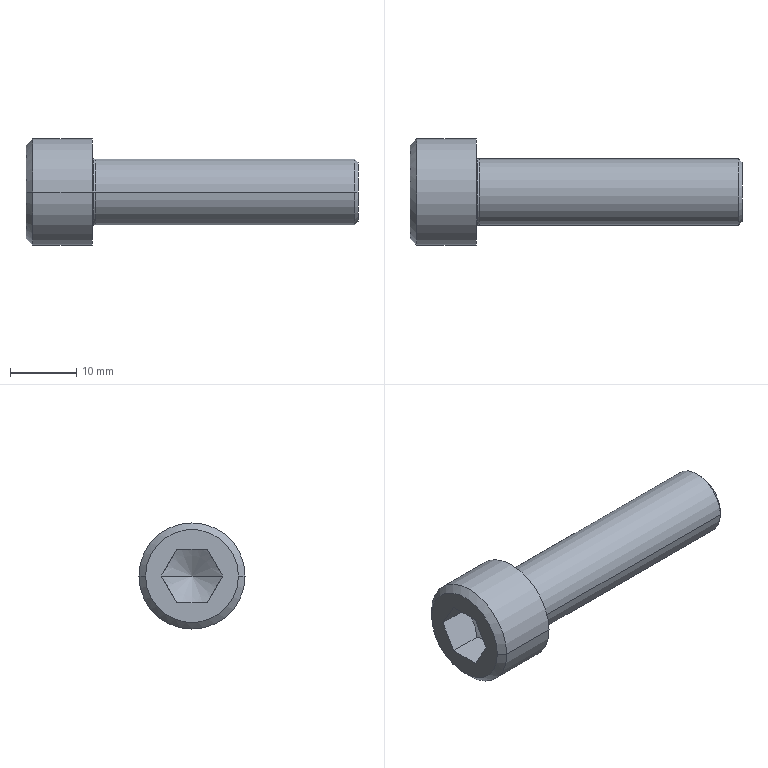Part | Creo | 1 solid | 23 faces | box 50 x 16 x 16 mm | volume 4790 mm3 | plane 9 | cone 6 | cylinder 4 | torus 4 | commonest cylinder face diameters 10 x2 16 x2
STEP:
#1=CARTESIAN_POINT('',(-308.5,10.376,-111.));
#2=VERTEX_POINT('',#1);
#3=CARTESIAN_POINT('',(-308.5,12.686,-107.));
#4=VERTEX_POINT('',#3);
#5=CARTESIAN_POINT('',(-308.5,10.376,-111.));
#6=CARTESIAN_POINT('',(-308.438,10.484,-110.814));
#7=CARTESIAN_POINT('',(-308.326,10.7,-110.439));
#8=CARTESIAN_POINT('',(-308.205,11.03,-109.869));
#9=CARTESIAN_POINT('',(-308.14,11.363,-109.291));
#10=CARTESIAN_POINT('',(-308.14,11.698,-108.712));
#11=CARTESIAN_POINT('',(-308.204,12.032,-108.133));
#12=CARTESIAN_POINT('',(-308.325,12.361,-107.563));
#13=CARTESIAN_POINT('',(-308.438,12.578,-107.187));
#14=CARTESIAN_POINT('',(-308.5,12.686,-107.));
#15=B_SPLINE_CURVE_WITH_KNOTS('',3,(#5,#6,#7,#8,#9,#10,#11,#12,#13,#14),.UNSPECIFIED.,.F.,.F.,(4,1,1,1,1,1,1,4),(0.,0.1429,0.2857,0.4286,0.5714,0.7143,0.8571,1.),.UNSPECIFIED.);
#16=EDGE_CURVE('',#2,#4,#15,.T.);
#17=ORIENTED_EDGE('',*,*,#16,.F.);
#18=CARTESIAN_POINT('',(-305.833,14.995,-111.));
#19=VERTEX_POINT('',#18);
#20=CARTESIAN_POINT('',(-305.833,14.995,-111.));
#21=DIRECTION('',(-0.5,-0.866,0.));
#22=VECTOR('',#21,5.333);
#23=LINE('',#20,#22);
#24=EDGE_CURVE('',#19,#2,#23,.T.);
#25=ORIENTED_EDGE('',*,*,#24,.F.);
#26=CARTESIAN_POINT('',(-308.5,19.614,-111.));
#27=VERTEX_POINT('',#26);
#28=CARTESIAN_POINT('',(-305.833,14.995,-111.));
#29=DIRECTION('',(-0.5,0.866,0.));
#30=VECTOR('',#29,5.333);
#31=LINE('',#28,#30);
#32=EDGE_CURVE('',#19,#27,#31,.T.);
#33=ORIENTED_EDGE('',*,*,#32,.T.);
#34=CARTESIAN_POINT('',(-308.5,17.305,-107.));
#35=VERTEX_POINT('',#34);
#36=CARTESIAN_POINT('',(-308.5,17.305,-107.));
#37=CARTESIAN_POINT('',(-308.438,17.412,-107.186));
#38=CARTESIAN_POINT('',(-308.326,17.628,-107.561));
#39=CARTESIAN_POINT('',(-308.205,17.958,-108.131));
#40=CARTESIAN_POINT('',(-308.14,18.291,-108.709));
#41=CARTESIAN_POINT('',(-308.14,18.626,-109.288));
#42=CARTESIAN_POINT('',(-308.204,18.96,-109.867));
#43=CARTESIAN_POINT('',(-308.325,19.289,-110.437));
#44=CARTESIAN_POINT('',(-308.438,19.506,-110.813));
#45=CARTESIAN_POINT('',(-308.5,19.614,-111.));
#46=B_SPLINE_CURVE_WITH_KNOTS('',3,(#36,#37,#38,#39,#40,#41,#42,#43,#44,#45),.UNSPECIFIED.,.F.,.F.,(4,1,1,1,1,1,1,4),(0.,0.1429,0.2857,0.4286,0.5714,0.7143,0.8571,1.),.UNSPECIFIED.);
#47=EDGE_CURVE('',#35,#27,#46,.T.);
#48=ORIENTED_EDGE('',*,*,#47,.F.);
#49=CARTESIAN_POINT('',(-308.5,12.686,-107.));
#50=CARTESIAN_POINT('',(-308.438,12.9,-107.));
#51=CARTESIAN_POINT('',(-308.327,13.33,-107.));
#52=CARTESIAN_POINT('',(-308.205,13.992,-107.));
#53=CARTESIAN_POINT('',(-308.14,14.66,-107.));
#54=CARTESIAN_POINT('',(-308.14,15.328,-107.));
#55=CARTESIAN_POINT('',(-308.204,15.996,-107.));
#56=CARTESIAN_POINT('',(-308.326,16.657,-107.));
#57=CARTESIAN_POINT('',(-308.438,17.09,-107.));
#58=CARTESIAN_POINT('',(-308.5,17.305,-107.));
#59=B_SPLINE_CURVE_WITH_KNOTS('',3,(#49,#50,#51,#52,#53,#54,#55,#56,#57,#58),.UNSPECIFIED.,.F.,.F.,(4,1,1,1,1,1,1,4),(0.,0.1429,0.2857,0.4286,0.5714,0.7143,0.8571,1.),.UNSPECIFIED.);
#60=EDGE_CURVE('',#4,#35,#59,.T.);
#61=ORIENTED_EDGE('',*,*,#60,.F.);
#62=EDGE_LOOP('',(#17,#25,#33,#48,#61));
#63=FACE_OUTER_BOUND('',#62,.F.);
#64=CARTESIAN_POINT('',(-307.193,14.995,-111.));
#65=DIRECTION('',(-1.,0.,0.));
#66=DIRECTION('',(0.,-1.,0.));
#67=AXIS2_PLACEMENT_3D('',#64,#65,#66);
#68=CONICAL_SURFACE('',#67,2.356,60.);
#69=ADVANCED_FACE('',(#63),#68,.F.);
#70=CARTESIAN_POINT('',(-313.5,12.686,-107.));
#71=VERTEX_POINT('',#70);
#72=CARTESIAN_POINT('',(-313.5,10.376,-111.));
#73=VERTEX_POINT('',#72);
#74=CARTESIAN_POINT('',(-313.5,12.686,-107.));
#75=DIRECTION('',(0.,-0.5,-0.866));
#76=VECTOR('',#75,4.619);
#77=LINE('',#74,#76);
#78=EDGE_CURVE('',#71,#73,#77,.T.);
#79=ORIENTED_EDGE('',*,*,#78,.T.);
#80=CARTESIAN_POINT('',(-313.5,10.376,-111.));
#81=DIRECTION('',(1.,0.,0.));
#82=VECTOR('',#81,5.);
#83=LINE('',#80,#82);
#84=EDGE_CURVE('',#73,#2,#83,.T.);
#85=ORIENTED_EDGE('',*,*,#84,.T.);
#86=ORIENTED_EDGE('',*,*,#16,.T.);
#87=CARTESIAN_POINT('',(-313.5,12.686,-107.));
#88=DIRECTION('',(1.,0.,0.));
#89=VECTOR('',#88,5.);
#90=LINE('',#87,#89);
#91=EDGE_CURVE('',#71,#4,#90,.T.);
#92=ORIENTED_EDGE('',*,*,#91,.F.);
#93=EDGE_LOOP('',(#79,#85,#86,#92));
#94=FACE_OUTER_BOUND('',#93,.F.);
#95=CARTESIAN_POINT('',(-308.5,12.686,-107.));
#96=DIRECTION('',(0.,0.866,-0.5));
#97=DIRECTION('',(0.,-0.5,-0.866));
#98=AXIS2_PLACEMENT_3D('',#95,#96,#97);
#99=PLANE('',#98);
#100=ADVANCED_FACE('',(#94),#99,.T.);
#101=CARTESIAN_POINT('',(-313.5,7.995,-111.));
#102=VERTEX_POINT('',#101);
#103=CARTESIAN_POINT('',(-313.5,21.995,-111.));
#104=VERTEX_POINT('',#103);
#105=CARTESIAN_POINT('',(-313.5,14.995,-111.));
#106=DIRECTION('',(-1.,0.,0.));
#107=DIRECTION('',(0.,-1.,0.));
#108=AXIS2_PLACEMENT_3D('',#105,#106,#107);
#109=CIRCLE('',#108,7.);
#110=EDGE_CURVE('',#102,#104,#109,.T.);
#111=ORIENTED_EDGE('',*,*,#110,.F.);
#112=CARTESIAN_POINT('',(-313.5,14.995,-111.));
#113=DIRECTION('',(-1.,0.,0.));
#114=DIRECTION('',(0.,1.,0.));
#115=AXIS2_PLACEMENT_3D('',#112,#113,#114);
#116=CIRCLE('',#115,7.);
#117=EDGE_CURVE('',#104,#102,#116,.T.);
#118=ORIENTED_EDGE('',*,*,#117,.F.);
#119=EDGE_LOOP('',(#111,#118));
#120=FACE_OUTER_BOUND('',#119,.F.);
#121=CARTESIAN_POINT('',(-313.5,12.686,-115.));
#122=VERTEX_POINT('',#121);
#123=CARTESIAN_POINT('',(-313.5,10.376,-111.));
#124=DIRECTION('',(0.,0.5,-0.866));
#125=VECTOR('',#124,4.619);
#126=LINE('',#123,#125);
#127=EDGE_CURVE('',#73,#122,#126,.T.);
#128=ORIENTED_EDGE('',*,*,#127,.F.);
#129=ORIENTED_EDGE('',*,*,#78,.F.);
#130=CARTESIAN_POINT('',(-313.5,17.305,-107.));
#131=VERTEX_POINT('',#130);
#132=CARTESIAN_POINT('',(-313.5,12.686,-107.));
#133=DIRECTION('',(0.,1.,0.));
#134=VECTOR('',#133,4.619);
#135=LINE('',#132,#134);
#136=EDGE_CURVE('',#71,#131,#135,.T.);
#137=ORIENTED_EDGE('',*,*,#136,.T.);
#138=CARTESIAN_POINT('',(-313.5,19.614,-111.));
#139=VERTEX_POINT('',#138);
#140=CARTESIAN_POINT('',(-313.5,19.614,-111.));
#141=DIRECTION('',(0.,-0.5,0.866));
#142=VECTOR('',#141,4.619);
#143=LINE('',#140,#142);
#144=EDGE_CURVE('',#139,#131,#143,.T.);
#145=ORIENTED_EDGE('',*,*,#144,.F.);
#146=CARTESIAN_POINT('',(-313.5,17.305,-115.));
#147=VERTEX_POINT('',#146);
#148=CARTESIAN_POINT('',(-313.5,17.305,-115.));
#149=DIRECTION('',(0.,0.5,0.866));
#150=VECTOR('',#149,4.619);
#151=LINE('',#148,#150);
#152=EDGE_CURVE('',#147,#139,#151,.T.);
#153=ORIENTED_EDGE('',*,*,#152,.F.);
#154=CARTESIAN_POINT('',(-313.5,17.305,-115.));
#155=DIRECTION('',(0.,-1.,0.));
#156=VECTOR('',#155,4.619);
#157=LINE('',#154,#156);
#158=EDGE_CURVE('',#147,#122,#157,.T.);
#159=ORIENTED_EDGE('',*,*,#158,.T.);
#160=EDGE_LOOP('',(#128,#129,#137,#145,#153,#159));
#161=FACE_BOUND('',#160,.F.);
#162=CARTESIAN_POINT('',(-313.5,14.995,-111.));
#163=DIRECTION('',(-1.,0.,0.));
#164=DIRECTION('',(0.,-1.,0.));
#165=AXIS2_PLACEMENT_3D('',#162,#163,#164);
#166=PLANE('',#165);
#167=ADVANCED_FACE('',(#120,#161),#166,.T.);
#168=CARTESIAN_POINT('',(-312.5,6.995,-111.));
#169=VERTEX_POINT('',#168);
#170=CARTESIAN_POINT('',(-312.5,22.995,-111.));
#171=VERTEX_POINT('',#170);
#172=CARTESIAN_POINT('',(-312.5,14.995,-111.));
#173=DIRECTION('',(-1.,0.,0.));
#174=DIRECTION('',(0.,-1.,0.));
#175=AXIS2_PLACEMENT_3D('',#172,#173,#174);
#176=CIRCLE('',#175,8.);
#177=EDGE_CURVE('',#169,#171,#176,.T.);
#178=ORIENTED_EDGE('',*,*,#177,.F.);
#179=CARTESIAN_POINT('',(-313.5,7.995,-111.));
#180=DIRECTION('',(0.7071,-0.7071,0.));
#181=VECTOR('',#180,1.414);
#182=LINE('',#179,#181);
#183=EDGE_CURVE('',#102,#169,#182,.T.);
#184=ORIENTED_EDGE('',*,*,#183,.F.);
#185=ORIENTED_EDGE('',*,*,#110,.T.);
#186=CARTESIAN_POINT('',(-313.5,21.995,-111.));
#187=DIRECTION('',(0.7071,0.7071,0.));
#188=VECTOR('',#187,1.414);
#189=LINE('',#186,#188);
#190=EDGE_CURVE('',#104,#171,#189,.T.);
#191=ORIENTED_EDGE('',*,*,#190,.T.);
#192=EDGE_LOOP('',(#178,#184,#185,#191));
#193=FACE_OUTER_BOUND('',#192,.F.);
#194=CARTESIAN_POINT('',(-313.,14.995,-111.));
#195=DIRECTION('',(1.,0.,0.));
#196=DIRECTION('',(0.,1.,0.));
#197=AXIS2_PLACEMENT_3D('',#194,#195,#196);
#198=CONICAL_SURFACE('',#197,7.5,45.);
#199=ADVANCED_FACE('',(#193),#198,.T.);
#200=ORIENTED_EDGE('',*,*,#177,.T.);
#201=CARTESIAN_POINT('',(-303.5,22.995,-111.));
#202=VERTEX_POINT('',#201);
#203=CARTESIAN_POINT('',(-303.5,22.995,-111.));
#204=DIRECTION('',(-1.,0.,0.));
#205=VECTOR('',#204,9.);
#206=LINE('',#203,#205);
#207=EDGE_CURVE('',#202,#171,#206,.T.);
#208=ORIENTED_EDGE('',*,*,#207,.F.);
#209=CARTESIAN_POINT('',(-303.5,6.995,-111.));
#210=VERTEX_POINT('',#209);
#211=CARTESIAN_POINT('',(-303.5,14.995,-111.));
#212=DIRECTION('',(1.,0.,0.));
#213=DIRECTION('',(0.,1.,0.));
#214=AXIS2_PLACEMENT_3D('',#211,#212,#213);
#215=CIRCLE('',#214,8.);
#216=EDGE_CURVE('',#202,#210,#215,.T.);
#217=ORIENTED_EDGE('',*,*,#216,.T.);
#218=CARTESIAN_POINT('',(-303.5,6.995,-111.));
#219=DIRECTION('',(-1.,0.,0.));
#220=VECTOR('',#219,9.);
#221=LINE('',#218,#220);
#222=EDGE_CURVE('',#210,#169,#221,.T.);
#223=ORIENTED_EDGE('',*,*,#222,.T.);
#224=EDGE_LOOP('',(#200,#208,#217,#223));
#225=FACE_OUTER_BOUND('',#224,.F.);
#226=CARTESIAN_POINT('',(-303.5,14.995,-111.));
#227=DIRECTION('',(-1.,0.,0.));
#228=DIRECTION('',(0.,-1.,0.));
#229=AXIS2_PLACEMENT_3D('',#226,#227,#228);
#230=CYLINDRICAL_SURFACE('',#229,8.);
#231=ADVANCED_FACE('',(#225),#230,.T.);
#232=CARTESIAN_POINT('',(-312.5,14.995,-111.));
#233=DIRECTION('',(-1.,0.,0.));
#234=DIRECTION('',(0.,1.,0.));
#235=AXIS2_PLACEMENT_3D('',#232,#233,#234);
#236=CIRCLE('',#235,8.);
#237=EDGE_CURVE('',#171,#169,#236,.T.);
#238=ORIENTED_EDGE('',*,*,#237,.T.);
#239=ORIENTED_EDGE('',*,*,#222,.F.);
#240=CARTESIAN_POINT('',(-303.5,14.995,-111.));
#241=DIRECTION('',(1.,0.,0.));
#242=DIRECTION('',(0.,-1.,0.));
#243=AXIS2_PLACEMENT_3D('',#240,#241,#242);
#244=CIRCLE('',#243,8.);
#245=EDGE_CURVE('',#210,#202,#244,.T.);
#246=ORIENTED_EDGE('',*,*,#245,.T.);
#247=ORIENTED_EDGE('',*,*,#207,.T.);
#248=EDGE_LOOP('',(#238,#239,#246,#247));
#249=FACE_OUTER_BOUND('',#248,.F.);
#250=CARTESIAN_POINT('',(-303.5,14.995,-111.));
#251=DIRECTION('',(-1.,0.,0.));
#252=DIRECTION('',(0.,-1.,0.));
#253=AXIS2_PLACEMENT_3D('',#250,#251,#252);
#254=CYLINDRICAL_SURFACE('',#253,8.);
#255=ADVANCED_FACE('',(#249),#254,.T.);
#256=ORIENTED_EDGE('',*,*,#237,.F.);
#257=ORIENTED_EDGE('',*,*,#190,.F.);
#258=ORIENTED_EDGE('',*,*,#117,.T.);
#259=ORIENTED_EDGE('',*,*,#183,.T.);
#260=EDGE_LOOP('',(#256,#257,#258,#259));
#261=FACE_OUTER_BOUND('',#260,.F.);
#262=CARTESIAN_POINT('',(-313.,14.995,-111.));
#263=DIRECTION('',(1.,0.,0.));
#264=DIRECTION('',(0.,1.,0.));
#265=AXIS2_PLACEMENT_3D('',#262,#263,#264);
#266=CONICAL_SURFACE('',#265,7.5,45.);
#267=ADVANCED_FACE('',(#261),#266,.T.);
#268=ORIENTED_EDGE('',*,*,#245,.F.);
#269=ORIENTED_EDGE('',*,*,#216,.F.);
#270=EDGE_LOOP('',(#268,#269));
#271=FACE_OUTER_BOUND('',#270,.F.);
#272=CARTESIAN_POINT('',(-303.5,9.595,-111.));
#273=VERTEX_POINT('',#272);
#274=CARTESIAN_POINT('',(-303.5,20.395,-111.));
#275=VERTEX_POINT('',#274);
#276=CARTESIAN_POINT('',(-303.5,14.995,-111.));
#277=DIRECTION('',(-1.,0.,0.));
#278=DIRECTION('',(0.,-1.,0.));
#279=AXIS2_PLACEMENT_3D('',#276,#277,#278);
#280=CIRCLE('',#279,5.4);
#281=EDGE_CURVE('',#273,#275,#280,.T.);
#282=ORIENTED_EDGE('',*,*,#281,.F.);
#283=CARTESIAN_POINT('',(-303.5,14.995,-111.));
#284=DIRECTION('',(-1.,0.,0.));
#285=DIRECTION('',(0.,1.,0.));
#286=AXIS2_PLACEMENT_3D('',#283,#284,#285);
#287=CIRCLE('',#286,5.4);
#288=EDGE_CURVE('',#275,#273,#287,.T.);
#289=ORIENTED_EDGE('',*,*,#288,.F.);
#290=EDGE_LOOP('',(#282,#289));
#291=FACE_BOUND('',#290,.F.);
#292=CARTESIAN_POINT('',(-303.5,14.995,-111.));
#293=DIRECTION('',(-1.,0.,0.));
#294=DIRECTION('',(0.,-1.,0.));
#295=AXIS2_PLACEMENT_3D('',#292,#293,#294);
#296=PLANE('',#295);
#297=ADVANCED_FACE('',(#271,#291),#296,.F.);
#298=ORIENTED_EDGE('',*,*,#281,.T.);
#299=CARTESIAN_POINT('',(-303.383,20.112,-111.));
#300=VERTEX_POINT('',#299);
#301=CARTESIAN_POINT('',(-303.1,20.395,-111.));
#302=DIRECTION('',(0.,0.,1.));
#303=DIRECTION('',(-1.,0.,0.));
#304=AXIS2_PLACEMENT_3D('',#301,#302,#303);
#305=CIRCLE('',#304,0.4);
#306=EDGE_CURVE('',#275,#300,#305,.T.);
#307=ORIENTED_EDGE('',*,*,#306,.T.);
#308=CARTESIAN_POINT('',(-303.383,9.878,-111.));
#309=VERTEX_POINT('',#308);
#310=CARTESIAN_POINT('',(-303.383,14.995,-111.));
#311=DIRECTION('',(-1.,0.,0.));
#312=DIRECTION('',(0.,-1.,0.));
#313=AXIS2_PLACEMENT_3D('',#310,#311,#312);
#314=CIRCLE('',#313,5.117);
#315=EDGE_CURVE('',#309,#300,#314,.T.);
#316=ORIENTED_EDGE('',*,*,#315,.F.);
#317=CARTESIAN_POINT('',(-303.1,9.595,-111.));
#318=DIRECTION('',(0.,0.,-1.));
#319=DIRECTION('',(-1.,0.,0.));
#320=AXIS2_PLACEMENT_3D('',#317,#318,#319);
#321=CIRCLE('',#320,0.4);
#322=EDGE_CURVE('',#273,#309,#321,.T.);
#323=ORIENTED_EDGE('',*,*,#322,.F.);
#324=EDGE_LOOP('',(#298,#307,#316,#323));
#325=FACE_OUTER_BOUND('',#324,.F.);
#326=CARTESIAN_POINT('',(-303.1,14.995,-111.));
#327=DIRECTION('',(-1.,0.,0.));
#328=DIRECTION('',(0.,-1.,0.));
#329=AXIS2_PLACEMENT_3D('',#326,#327,#328);
#330=TOROIDAL_SURFACE('',#329,5.4,0.4);
#331=ADVANCED_FACE('',(#325),#330,.F.);
#332=ORIENTED_EDGE('',*,*,#288,.T.);
#333=ORIENTED_EDGE('',*,*,#322,.T.);
#334=CARTESIAN_POINT('',(-303.383,14.995,-111.));
#335=DIRECTION('',(-1.,0.,0.));
#336=DIRECTION('',(0.,1.,0.));
#337=AXIS2_PLACEMENT_3D('',#334,#335,#336);
#338=CIRCLE('',#337,5.117);
#339=EDGE_CURVE('',#300,#309,#338,.T.);
#340=ORIENTED_EDGE('',*,*,#339,.F.);
#341=ORIENTED_EDGE('',*,*,#306,.F.);
#342=EDGE_LOOP('',(#332,#333,#340,#341));
#343=FACE_OUTER_BOUND('',#342,.F.);
#344=CARTESIAN_POINT('',(-303.1,14.995,-111.));
#345=DIRECTION('',(-1.,0.,0.));
#346=DIRECTION('',(0.,-1.,0.));
#347=AXIS2_PLACEMENT_3D('',#344,#345,#346);
#348=TOROIDAL_SURFACE('',#347,5.4,0.4);
#349=ADVANCED_FACE('',(#343),#348,.F.);
#350=CARTESIAN_POINT('',(-303.1,19.995,-111.));
#351=VERTEX_POINT('',#350);
#352=CARTESIAN_POINT('',(-303.1,9.995,-111.));
#353=VERTEX_POINT('',#352);
#354=CARTESIAN_POINT('',(-303.1,14.995,-111.));
#355=DIRECTION('',(-1.,0.,0.));
#356=DIRECTION('',(0.,1.,0.));
#357=AXIS2_PLACEMENT_3D('',#354,#355,#356);
#358=CIRCLE('',#357,5.);
#359=EDGE_CURVE('',#351,#353,#358,.T.);
#360=ORIENTED_EDGE('',*,*,#359,.F.);
#361=CARTESIAN_POINT('',(-303.1,20.395,-111.));
#362=DIRECTION('',(0.,0.,1.));
#363=DIRECTION('',(-0.7071,-0.7071,0.));
#364=AXIS2_PLACEMENT_3D('',#361,#362,#363);
#365=CIRCLE('',#364,0.4);
#366=EDGE_CURVE('',#300,#351,#365,.T.);
#367=ORIENTED_EDGE('',*,*,#366,.F.);
#368=ORIENTED_EDGE('',*,*,#339,.T.);
#369=CARTESIAN_POINT('',(-303.1,9.595,-111.));
#370=DIRECTION('',(0.,0.,-1.));
#371=DIRECTION('',(-0.7071,0.7071,0.));
#372=AXIS2_PLACEMENT_3D('',#369,#370,#371);
#373=CIRCLE('',#372,0.4);
#374=EDGE_CURVE('',#309,#353,#373,.T.);
#375=ORIENTED_EDGE('',*,*,#374,.T.);
#376=EDGE_LOOP('',(#360,#367,#368,#375));
#377=FACE_OUTER_BOUND('',#376,.F.);
#378=CARTESIAN_POINT('',(-303.1,14.995,-111.));
#379=DIRECTION('',(-1.,0.,0.));
#380=DIRECTION('',(0.,-1.,0.));
#381=AXIS2_PLACEMENT_3D('',#378,#379,#380);
#382=TOROIDAL_SURFACE('',#381,5.4,0.4);
#383=ADVANCED_FACE('',(#377),#382,.F.);
#384=CARTESIAN_POINT('',(-264.,9.995,-111.));
#385=VERTEX_POINT('',#384);
#386=CARTESIAN_POINT('',(-264.,19.995,-111.));
#387=VERTEX_POINT('',#386);
#388=CARTESIAN_POINT('',(-264.,14.995,-111.));
#389=DIRECTION('',(1.,0.,0.));
#390=DIRECTION('',(0.,-1.,0.));
#391=AXIS2_PLACEMENT_3D('',#388,#389,#390);
#392=CIRCLE('',#391,5.);
#393=EDGE_CURVE('',#385,#387,#392,.T.);
#394=ORIENTED_EDGE('',*,*,#393,.T.);
#395=CARTESIAN_POINT('',(-264.,19.995,-111.));
#396=DIRECTION('',(-1.,0.,0.));
#397=VECTOR('',#396,39.1);
#398=LINE('',#395,#397);
#399=EDGE_CURVE('',#387,#351,#398,.T.);
#400=ORIENTED_EDGE('',*,*,#399,.T.);
#401=ORIENTED_EDGE('',*,*,#359,.T.);
#402=CARTESIAN_POINT('',(-264.,9.995,-111.));
#403=DIRECTION('',(-1.,0.,0.));
#404=VECTOR('',#403,39.1);
#405=LINE('',#402,#404);
#406=EDGE_CURVE('',#385,#353,#405,.T.);
#407=ORIENTED_EDGE('',*,*,#406,.F.);
#408=EDGE_LOOP('',(#394,#400,#401,#407));
#409=FACE_OUTER_BOUND('',#408,.F.);
#410=CARTESIAN_POINT('',(-263.5,14.995,-111.));
#411=DIRECTION('',(-1.,0.,0.));
#412=DIRECTION('',(0.,-1.,0.));
#413=AXIS2_PLACEMENT_3D('',#410,#411,#412);
#414=CYLINDRICAL_SURFACE('',#413,5.);
#415=ADVANCED_FACE('',(#409),#414,.T.);
#416=CARTESIAN_POINT('',(-263.5,10.495,-111.));
#417=VERTEX_POINT('',#416);
#418=CARTESIAN_POINT('',(-263.5,19.495,-111.));
#419=VERTEX_POINT('',#418);
#420=CARTESIAN_POINT('',(-263.5,14.995,-111.));
#421=DIRECTION('',(1.,0.,0.));
#422=DIRECTION('',(0.,-1.,0.));
#423=AXIS2_PLACEMENT_3D('',#420,#421,#422);
#424=CIRCLE('',#423,4.5);
#425=EDGE_CURVE('',#417,#419,#424,.T.);
#426=ORIENTED_EDGE('',*,*,#425,.T.);
#427=CARTESIAN_POINT('',(-263.5,19.495,-111.));
#428=DIRECTION('',(-0.7071,0.7071,0.));
#429=VECTOR('',#428,0.7071);
#430=LINE('',#427,#429);
#431=EDGE_CURVE('',#419,#387,#430,.T.);
#432=ORIENTED_EDGE('',*,*,#431,.T.);
#433=ORIENTED_EDGE('',*,*,#393,.F.);
#434=CARTESIAN_POINT('',(-263.5,10.495,-111.));
#435=DIRECTION('',(-0.7071,-0.7071,0.));
#436=VECTOR('',#435,0.7071);
#437=LINE('',#434,#436);
#438=EDGE_CURVE('',#417,#385,#437,.T.);
#439=ORIENTED_EDGE('',*,*,#438,.F.);
#440=EDGE_LOOP('',(#426,#432,#433,#439));
#441=FACE_OUTER_BOUND('',#440,.F.);
#442=CARTESIAN_POINT('',(-263.75,14.995,-111.));
#443=DIRECTION('',(-1.,0.,0.));
#444=DIRECTION('',(0.,-1.,0.));
#445=AXIS2_PLACEMENT_3D('',#442,#443,#444);
#446=CONICAL_SURFACE('',#445,4.75,45.);
#447=ADVANCED_FACE('',(#441),#446,.T.);
#448=ORIENTED_EDGE('',*,*,#425,.F.);
#449=CARTESIAN_POINT('',(-263.5,14.995,-111.));
#450=DIRECTION('',(1.,0.,0.));
#451=DIRECTION('',(0.,1.,0.));
#452=AXIS2_PLACEMENT_3D('',#449,#450,#451);
#453=CIRCLE('',#452,4.5);
#454=EDGE_CURVE('',#419,#417,#453,.T.);
#455=ORIENTED_EDGE('',*,*,#454,.F.);
#456=EDGE_LOOP('',(#448,#455));
#457=FACE_OUTER_BOUND('',#456,.F.);
#458=CARTESIAN_POINT('',(-263.5,14.995,-111.));
#459=DIRECTION('',(-1.,0.,0.));
#460=DIRECTION('',(0.,-1.,0.));
#461=AXIS2_PLACEMENT_3D('',#458,#459,#460);
#462=PLANE('',#461);
#463=ADVANCED_FACE('',(#457),#462,.F.);
#464=ORIENTED_EDGE('',*,*,#454,.T.);
#465=ORIENTED_EDGE('',*,*,#438,.T.);
#466=CARTESIAN_POINT('',(-264.,14.995,-111.));
#467=DIRECTION('',(1.,0.,0.));
#468=DIRECTION('',(0.,1.,0.));
#469=AXIS2_PLACEMENT_3D('',#466,#467,#468);
#470=CIRCLE('',#469,5.);
#471=EDGE_CURVE('',#387,#385,#470,.T.);
#472=ORIENTED_EDGE('',*,*,#471,.F.);
#473=ORIENTED_EDGE('',*,*,#431,.F.);
#474=EDGE_LOOP('',(#464,#465,#472,#473));
#475=FACE_OUTER_BOUND('',#474,.F.);
#476=CARTESIAN_POINT('',(-263.75,14.995,-111.));
#477=DIRECTION('',(-1.,0.,0.));
#478=DIRECTION('',(0.,-1.,0.));
#479=AXIS2_PLACEMENT_3D('',#476,#477,#478);
#480=CONICAL_SURFACE('',#479,4.75,45.);
#481=ADVANCED_FACE('',(#475),#480,.T.);
#482=ORIENTED_EDGE('',*,*,#471,.T.);
#483=ORIENTED_EDGE('',*,*,#406,.T.);
#484=CARTESIAN_POINT('',(-303.1,14.995,-111.));
#485=DIRECTION('',(-1.,0.,0.));
#486=DIRECTION('',(0.,-1.,0.));
#487=AXIS2_PLACEMENT_3D('',#484,#485,#486);
#488=CIRCLE('',#487,5.);
#489=EDGE_CURVE('',#353,#351,#488,.T.);
#490=ORIENTED_EDGE('',*,*,#489,.T.);
#491=ORIENTED_EDGE('',*,*,#399,.F.);
#492=EDGE_LOOP('',(#482,#483,#490,#491));
#493=FACE_OUTER_BOUND('',#492,.F.);
#494=CARTESIAN_POINT('',(-263.5,14.995,-111.));
#495=DIRECTION('',(-1.,0.,0.));
#496=DIRECTION('',(0.,-1.,0.));
#497=AXIS2_PLACEMENT_3D('',#494,#495,#496);
#498=CYLINDRICAL_SURFACE('',#497,5.);
#499=ADVANCED_FACE('',(#493),#498,.T.);
#500=ORIENTED_EDGE('',*,*,#489,.F.);
#501=ORIENTED_EDGE('',*,*,#374,.F.);
#502=ORIENTED_EDGE('',*,*,#315,.T.);
#503=ORIENTED_EDGE('',*,*,#366,.T.);
#504=EDGE_LOOP('',(#500,#501,#502,#503));
#505=FACE_OUTER_BOUND('',#504,.F.);
#506=CARTESIAN_POINT('',(-303.1,14.995,-111.));
#507=DIRECTION('',(-1.,0.,0.));
#508=DIRECTION('',(0.,-1.,0.));
#509=AXIS2_PLACEMENT_3D('',#506,#507,#508);
#510=TOROIDAL_SURFACE('',#509,5.4,0.4);
#511=ADVANCED_FACE('',(#505),#510,.F.);
#512=ORIENTED_EDGE('',*,*,#127,.T.);
#513=CARTESIAN_POINT('',(-308.5,12.686,-115.));
#514=VERTEX_POINT('',#513);
#515=CARTESIAN_POINT('',(-313.5,12.686,-115.));
#516=DIRECTION('',(1.,0.,0.));
#517=VECTOR('',#516,5.);
#518=LINE('',#515,#517);
#519=EDGE_CURVE('',#122,#514,#518,.T.);
#520=ORIENTED_EDGE('',*,*,#519,.T.);
#521=CARTESIAN_POINT('',(-308.5,12.686,-115.));
#522=CARTESIAN_POINT('',(-308.438,12.578,-114.814));
#523=CARTESIAN_POINT('',(-308.326,12.362,-114.439));
#524=CARTESIAN_POINT('',(-308.205,12.033,-113.869));
#525=CARTESIAN_POINT('',(-308.14,11.699,-113.291));
#526=CARTESIAN_POINT('',(-308.14,11.365,-112.712));
#527=CARTESIAN_POINT('',(-308.204,11.031,-112.133));
#528=CARTESIAN_POINT('',(-308.325,10.701,-111.563));
#529=CARTESIAN_POINT('',(-308.438,10.485,-111.187));
#530=CARTESIAN_POINT('',(-308.5,10.376,-111.));
#531=B_SPLINE_CURVE_WITH_KNOTS('',3,(#521,#522,#523,#524,#525,#526,#527,#528,#529,#530),.UNSPECIFIED.,.F.,.F.,(4,1,1,1,1,1,1,4),(0.,0.1429,0.2857,0.4286,0.5714,0.7143,0.8571,1.),.UNSPECIFIED.);
#532=EDGE_CURVE('',#514,#2,#531,.T.);
#533=ORIENTED_EDGE('',*,*,#532,.T.);
#534=ORIENTED_EDGE('',*,*,#84,.F.);
#535=EDGE_LOOP('',(#512,#520,#533,#534));
#536=FACE_OUTER_BOUND('',#535,.F.);
#537=CARTESIAN_POINT('',(-308.5,10.376,-111.));
#538=DIRECTION('',(0.,0.866,0.5));
#539=DIRECTION('',(0.,0.5,-0.866));
#540=AXIS2_PLACEMENT_3D('',#537,#538,#539);
#541=PLANE('',#540);
#542=ADVANCED_FACE('',(#536),#541,.T.);
#543=ORIENTED_EDGE('',*,*,#158,.F.);
#544=CARTESIAN_POINT('',(-308.5,17.305,-115.));
#545=VERTEX_POINT('',#544);
#546=CARTESIAN_POINT('',(-313.5,17.305,-115.));
#547=DIRECTION('',(1.,0.,0.));
#548=VECTOR('',#547,5.);
#549=LINE('',#546,#548);
#550=EDGE_CURVE('',#147,#545,#549,.T.);
#551=ORIENTED_EDGE('',*,*,#550,.T.);
#552=CARTESIAN_POINT('',(-308.5,17.305,-115.));
#553=CARTESIAN_POINT('',(-308.438,17.09,-115.));
#554=CARTESIAN_POINT('',(-308.326,16.657,-115.));
#555=CARTESIAN_POINT('',(-308.204,15.996,-115.));
#556=CARTESIAN_POINT('',(-308.14,15.328,-115.));
#557=CARTESIAN_POINT('',(-308.14,14.66,-115.));
#558=CARTESIAN_POINT('',(-308.205,13.992,-115.));
#559=CARTESIAN_POINT('',(-308.327,13.33,-115.));
#560=CARTESIAN_POINT('',(-308.438,12.9,-115.));
#561=CARTESIAN_POINT('',(-308.5,12.686,-115.));
#562=B_SPLINE_CURVE_WITH_KNOTS('',3,(#552,#553,#554,#555,#556,#557,#558,#559,#560,#561),.UNSPECIFIED.,.F.,.F.,(4,1,1,1,1,1,1,4),(0.,0.1429,0.2857,0.4286,0.5714,0.7143,0.8571,1.),.UNSPECIFIED.);
#563=EDGE_CURVE('',#545,#514,#562,.T.);
#564=ORIENTED_EDGE('',*,*,#563,.T.);
#565=ORIENTED_EDGE('',*,*,#519,.F.);
#566=EDGE_LOOP('',(#543,#551,#564,#565));
#567=FACE_OUTER_BOUND('',#566,.F.);
#568=CARTESIAN_POINT('',(-308.5,12.686,-115.));
#569=DIRECTION('',(0.,0.,1.));
#570=DIRECTION('',(-1.,0.,0.));
#571=AXIS2_PLACEMENT_3D('',#568,#569,#570);
#572=PLANE('',#571);
#573=ADVANCED_FACE('',(#567),#572,.T.);
#574=ORIENTED_EDGE('',*,*,#152,.T.);
#575=CARTESIAN_POINT('',(-313.5,19.614,-111.));
#576=DIRECTION('',(1.,0.,0.));
#577=VECTOR('',#576,5.);
#578=LINE('',#575,#577);
#579=EDGE_CURVE('',#139,#27,#578,.T.);
#580=ORIENTED_EDGE('',*,*,#579,.T.);
#581=CARTESIAN_POINT('',(-308.5,19.614,-111.));
#582=CARTESIAN_POINT('',(-308.438,19.506,-111.187));
#583=CARTESIAN_POINT('',(-308.325,19.289,-111.563));
#584=CARTESIAN_POINT('',(-308.204,18.96,-112.133));
#585=CARTESIAN_POINT('',(-308.14,18.626,-112.712));
#586=CARTESIAN_POINT('',(-308.14,18.291,-113.291));
#587=CARTESIAN_POINT('',(-308.205,17.958,-113.869));
#588=CARTESIAN_POINT('',(-308.326,17.628,-114.439));
#589=CARTESIAN_POINT('',(-308.438,17.412,-114.814));
#590=CARTESIAN_POINT('',(-308.5,17.305,-115.));
#591=B_SPLINE_CURVE_WITH_KNOTS('',3,(#581,#582,#583,#584,#585,#586,#587,#588,#589,#590),.UNSPECIFIED.,.F.,.F.,(4,1,1,1,1,1,1,4),(0.,0.1429,0.2857,0.4286,0.5714,0.7143,0.8571,1.),.UNSPECIFIED.);
#592=EDGE_CURVE('',#27,#545,#591,.T.);
#593=ORIENTED_EDGE('',*,*,#592,.T.);
#594=ORIENTED_EDGE('',*,*,#550,.F.);
#595=EDGE_LOOP('',(#574,#580,#593,#594));
#596=FACE_OUTER_BOUND('',#595,.F.);
#597=CARTESIAN_POINT('',(-308.5,17.305,-115.));
#598=DIRECTION('',(0.,-0.866,0.5));
#599=DIRECTION('',(0.,0.5,0.866));
#600=AXIS2_PLACEMENT_3D('',#597,#598,#599);
#601=PLANE('',#600);
#602=ADVANCED_FACE('',(#596),#601,.T.);
#603=ORIENTED_EDGE('',*,*,#144,.T.);
#604=CARTESIAN_POINT('',(-313.5,17.305,-107.));
#605=DIRECTION('',(1.,0.,0.));
#606=VECTOR('',#605,5.);
#607=LINE('',#604,#606);
#608=EDGE_CURVE('',#131,#35,#607,.T.);
#609=ORIENTED_EDGE('',*,*,#608,.T.);
#610=ORIENTED_EDGE('',*,*,#47,.T.);
#611=ORIENTED_EDGE('',*,*,#579,.F.);
#612=EDGE_LOOP('',(#603,#609,#610,#611));
#613=FACE_OUTER_BOUND('',#612,.F.);
#614=CARTESIAN_POINT('',(-308.5,19.614,-111.));
#615=DIRECTION('',(0.,-0.866,-0.5));
#616=DIRECTION('',(0.,-0.5,0.866));
#617=AXIS2_PLACEMENT_3D('',#614,#615,#616);
#618=PLANE('',#617);
#619=ADVANCED_FACE('',(#613),#618,.T.);
#620=ORIENTED_EDGE('',*,*,#136,.F.);
#621=ORIENTED_EDGE('',*,*,#91,.T.);
#622=ORIENTED_EDGE('',*,*,#60,.T.);
#623=ORIENTED_EDGE('',*,*,#608,.F.);
#624=EDGE_LOOP('',(#620,#621,#622,#623));
#625=FACE_OUTER_BOUND('',#624,.F.);
#626=CARTESIAN_POINT('',(-308.5,17.305,-107.));
#627=DIRECTION('',(0.,0.,-1.));
#628=DIRECTION('',(1.,0.,0.));
#629=AXIS2_PLACEMENT_3D('',#626,#627,#628);
#630=PLANE('',#629);
#631=ADVANCED_FACE('',(#625),#630,.T.);
#632=ORIENTED_EDGE('',*,*,#592,.F.);
#633=ORIENTED_EDGE('',*,*,#32,.F.);
#634=ORIENTED_EDGE('',*,*,#24,.T.);
#635=ORIENTED_EDGE('',*,*,#532,.F.);
#636=ORIENTED_EDGE('',*,*,#563,.F.);
#637=EDGE_LOOP('',(#632,#633,#634,#635,#636));
#638=FACE_OUTER_BOUND('',#637,.F.);
#639=CARTESIAN_POINT('',(-307.193,14.995,-111.));
#640=DIRECTION('',(-1.,0.,0.));
#641=DIRECTION('',(0.,-1.,0.));
#642=AXIS2_PLACEMENT_3D('',#639,#640,#641);
#643=CONICAL_SURFACE('',#642,2.356,60.);
#644=ADVANCED_FACE('',(#638),#643,.F.);
#645=CLOSED_SHELL('',(#69,#100,#167,#199,#231,#255,#267,#297,#331,#349,#383,#415,#447,#463,#481,#499,#511,#542,#573,#602,#619,#631,#644));
#646=MANIFOLD_SOLID_BREP('',#645);
#647=(LENGTH_UNIT()NAMED_UNIT(*)SI_UNIT(.MILLI.,.METRE.));
#648=UNCERTAINTY_MEASURE_WITH_UNIT(LENGTH_MEASURE(0.005488),#647,'','');
#649=(NAMED_UNIT(*)PLANE_ANGLE_UNIT()SI_UNIT($,.RADIAN.));
#650=PLANE_ANGLE_MEASURE_WITH_UNIT(PLANE_ANGLE_MEASURE(0.01745),#649);
#651=(CONVERSION_BASED_UNIT('DEGREE',#650)NAMED_UNIT(*)PLANE_ANGLE_UNIT());
#652=(NAMED_UNIT(*)SI_UNIT($,.STERADIAN.)SOLID_ANGLE_UNIT());
#653=(GEOMETRIC_REPRESENTATION_CONTEXT(3)GLOBAL_UNCERTAINTY_ASSIGNED_CONTEXT((#648))GLOBAL_UNIT_ASSIGNED_CONTEXT((#647,#651,#652))REPRESENTATION_CONTEXT('',''));
#654=ADVANCED_BREP_SHAPE_REPRESENTATION('',(#646),#653);